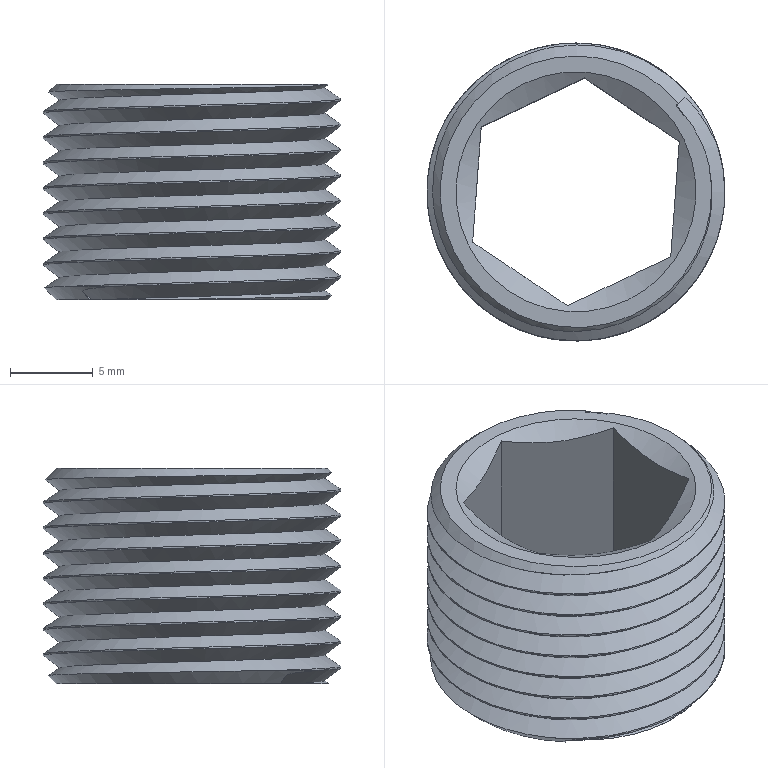Part | NX | features BREP 1 | 1 solid | 22 faces | box 18 x 18 x 13 mm | volume 1322 mm3 | plane 16 | cone 3 | spline 2 | cylinder 1 | commonest cylinder face diameters 18 x1